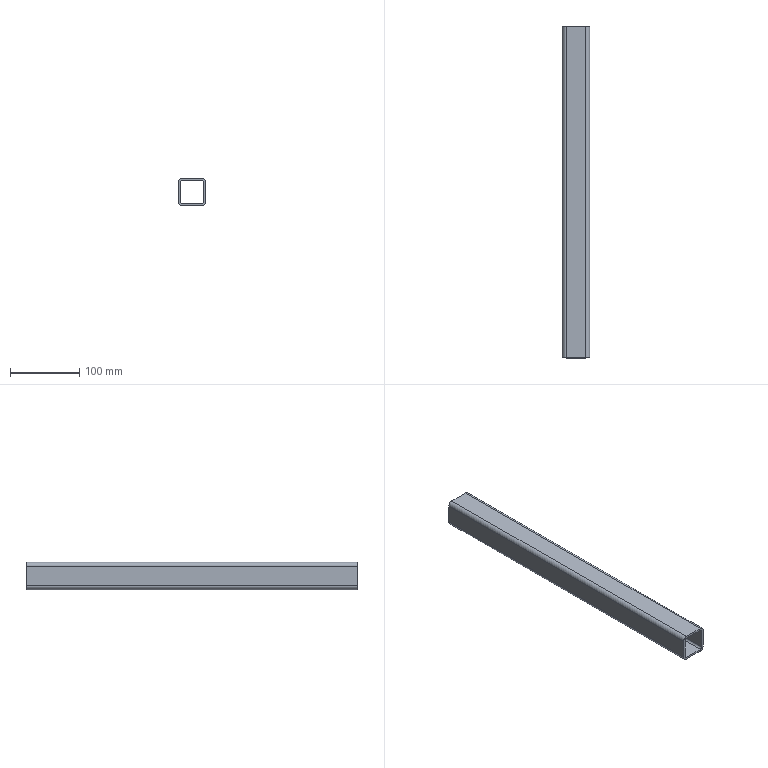Part | SolidWorks | features WeldMemberFeat 1, WeldmentFeature 1 | 1 solid | 18 faces | box 40 x 480 x 40 mm | volume 201995 mm3 | plane 10 | cylinder 8 | commonest cylinder face diameters 6 x4 12 x4
STEP:
#1=CARTESIAN_POINT('',(-20.,0.,14.));
#2=VERTEX_POINT('',#1);
#3=CARTESIAN_POINT('',(-14.,0.,20.));
#4=VERTEX_POINT('',#3);
#5=CARTESIAN_POINT('',(-14.,0.,14.));
#6=DIRECTION('',(0.,1.,0.));
#7=DIRECTION('',(0.,0.,1.));
#8=AXIS2_PLACEMENT_3D('',#5,#6,#7);
#9=CIRCLE('',#8,6.);
#10=EDGE_CURVE('',#2,#4,#9,.T.);
#11=ORIENTED_EDGE('',*,*,#10,.T.);
#12=CARTESIAN_POINT('',(-14.,480.,20.));
#13=VERTEX_POINT('',#12);
#14=CARTESIAN_POINT('',(-14.,480.,20.));
#15=DIRECTION('',(0.,-1.,0.));
#16=VECTOR('',#15,1000.);
#17=LINE('',#14,#16);
#18=EDGE_CURVE('',#13,#4,#17,.T.);
#19=ORIENTED_EDGE('',*,*,#18,.F.);
#20=CARTESIAN_POINT('',(-20.,480.,14.));
#21=VERTEX_POINT('',#20);
#22=CARTESIAN_POINT('',(-14.,480.,14.));
#23=DIRECTION('',(0.,1.,0.));
#24=DIRECTION('',(0.,0.,1.));
#25=AXIS2_PLACEMENT_3D('',#22,#23,#24);
#26=CIRCLE('',#25,6.);
#27=EDGE_CURVE('',#21,#13,#26,.T.);
#28=ORIENTED_EDGE('',*,*,#27,.F.);
#29=CARTESIAN_POINT('',(-20.,480.,14.));
#30=DIRECTION('',(0.,-1.,0.));
#31=VECTOR('',#30,1000.);
#32=LINE('',#29,#31);
#33=EDGE_CURVE('',#21,#2,#32,.T.);
#34=ORIENTED_EDGE('',*,*,#33,.T.);
#35=EDGE_LOOP('',(#11,#19,#28,#34));
#36=FACE_OUTER_BOUND('',#35,.T.);
#37=CARTESIAN_POINT('',(-14.,480.,14.));
#38=DIRECTION('',(0.,-1.,0.));
#39=DIRECTION('',(0.,0.,-1.));
#40=AXIS2_PLACEMENT_3D('',#37,#38,#39);
#41=CYLINDRICAL_SURFACE('',#40,6.);
#42=ADVANCED_FACE('',(#36),#41,.T.);
#43=CARTESIAN_POINT('',(14.,0.,20.));
#44=VERTEX_POINT('',#43);
#45=CARTESIAN_POINT('',(-14.,0.,20.));
#46=DIRECTION('',(1.,0.,0.));
#47=VECTOR('',#46,1000.);
#48=LINE('',#45,#47);
#49=EDGE_CURVE('',#4,#44,#48,.T.);
#50=ORIENTED_EDGE('',*,*,#49,.T.);
#51=CARTESIAN_POINT('',(14.,480.,20.));
#52=VERTEX_POINT('',#51);
#53=CARTESIAN_POINT('',(14.,480.,20.));
#54=DIRECTION('',(0.,-1.,0.));
#55=VECTOR('',#54,1000.);
#56=LINE('',#53,#55);
#57=EDGE_CURVE('',#52,#44,#56,.T.);
#58=ORIENTED_EDGE('',*,*,#57,.F.);
#59=CARTESIAN_POINT('',(-14.,480.,20.));
#60=DIRECTION('',(1.,0.,0.));
#61=VECTOR('',#60,1000.);
#62=LINE('',#59,#61);
#63=EDGE_CURVE('',#13,#52,#62,.T.);
#64=ORIENTED_EDGE('',*,*,#63,.F.);
#65=ORIENTED_EDGE('',*,*,#18,.T.);
#66=EDGE_LOOP('',(#50,#58,#64,#65));
#67=FACE_OUTER_BOUND('',#66,.T.);
#68=CARTESIAN_POINT('',(-14.,480.,20.));
#69=DIRECTION('',(0.,0.,-1.));
#70=DIRECTION('',(-1.,0.,0.));
#71=AXIS2_PLACEMENT_3D('',#68,#69,#70);
#72=PLANE('',#71);
#73=ADVANCED_FACE('',(#67),#72,.F.);
#74=CARTESIAN_POINT('',(20.,0.,14.));
#75=VERTEX_POINT('',#74);
#76=CARTESIAN_POINT('',(14.,0.,14.));
#77=DIRECTION('',(0.,1.,0.));
#78=DIRECTION('',(0.,0.,1.));
#79=AXIS2_PLACEMENT_3D('',#76,#77,#78);
#80=CIRCLE('',#79,6.);
#81=EDGE_CURVE('',#44,#75,#80,.T.);
#82=ORIENTED_EDGE('',*,*,#81,.T.);
#83=CARTESIAN_POINT('',(20.,480.,14.));
#84=VERTEX_POINT('',#83);
#85=CARTESIAN_POINT('',(20.,480.,14.));
#86=DIRECTION('',(0.,-1.,0.));
#87=VECTOR('',#86,1000.);
#88=LINE('',#85,#87);
#89=EDGE_CURVE('',#84,#75,#88,.T.);
#90=ORIENTED_EDGE('',*,*,#89,.F.);
#91=CARTESIAN_POINT('',(14.,480.,14.));
#92=DIRECTION('',(0.,1.,0.));
#93=DIRECTION('',(0.,0.,1.));
#94=AXIS2_PLACEMENT_3D('',#91,#92,#93);
#95=CIRCLE('',#94,6.);
#96=EDGE_CURVE('',#52,#84,#95,.T.);
#97=ORIENTED_EDGE('',*,*,#96,.F.);
#98=ORIENTED_EDGE('',*,*,#57,.T.);
#99=EDGE_LOOP('',(#82,#90,#97,#98));
#100=FACE_OUTER_BOUND('',#99,.T.);
#101=CARTESIAN_POINT('',(14.,480.,14.));
#102=DIRECTION('',(0.,-1.,0.));
#103=DIRECTION('',(0.,0.,-1.));
#104=AXIS2_PLACEMENT_3D('',#101,#102,#103);
#105=CYLINDRICAL_SURFACE('',#104,6.);
#106=ADVANCED_FACE('',(#100),#105,.T.);
#107=CARTESIAN_POINT('',(20.,0.,-14.));
#108=VERTEX_POINT('',#107);
#109=CARTESIAN_POINT('',(20.,0.,-14.));
#110=DIRECTION('',(0.,0.,-1.));
#111=VECTOR('',#110,1000.);
#112=LINE('',#109,#111);
#113=EDGE_CURVE('',#75,#108,#112,.T.);
#114=ORIENTED_EDGE('',*,*,#113,.T.);
#115=CARTESIAN_POINT('',(20.,480.,-14.));
#116=VERTEX_POINT('',#115);
#117=CARTESIAN_POINT('',(20.,480.,-14.));
#118=DIRECTION('',(0.,-1.,0.));
#119=VECTOR('',#118,1000.);
#120=LINE('',#117,#119);
#121=EDGE_CURVE('',#116,#108,#120,.T.);
#122=ORIENTED_EDGE('',*,*,#121,.F.);
#123=CARTESIAN_POINT('',(20.,480.,-14.));
#124=DIRECTION('',(0.,0.,-1.));
#125=VECTOR('',#124,1000.);
#126=LINE('',#123,#125);
#127=EDGE_CURVE('',#84,#116,#126,.T.);
#128=ORIENTED_EDGE('',*,*,#127,.F.);
#129=ORIENTED_EDGE('',*,*,#89,.T.);
#130=EDGE_LOOP('',(#114,#122,#128,#129));
#131=FACE_OUTER_BOUND('',#130,.T.);
#132=CARTESIAN_POINT('',(20.,480.,-14.));
#133=DIRECTION('',(-1.,0.,0.));
#134=DIRECTION('',(0.,0.,1.));
#135=AXIS2_PLACEMENT_3D('',#132,#133,#134);
#136=PLANE('',#135);
#137=ADVANCED_FACE('',(#131),#136,.F.);
#138=CARTESIAN_POINT('',(14.,0.,-20.));
#139=VERTEX_POINT('',#138);
#140=CARTESIAN_POINT('',(14.,0.,-14.));
#141=DIRECTION('',(0.,1.,0.));
#142=DIRECTION('',(0.,0.,1.));
#143=AXIS2_PLACEMENT_3D('',#140,#141,#142);
#144=CIRCLE('',#143,6.);
#145=EDGE_CURVE('',#108,#139,#144,.T.);
#146=ORIENTED_EDGE('',*,*,#145,.T.);
#147=CARTESIAN_POINT('',(14.,480.,-20.));
#148=VERTEX_POINT('',#147);
#149=CARTESIAN_POINT('',(14.,480.,-20.));
#150=DIRECTION('',(0.,-1.,0.));
#151=VECTOR('',#150,1000.);
#152=LINE('',#149,#151);
#153=EDGE_CURVE('',#148,#139,#152,.T.);
#154=ORIENTED_EDGE('',*,*,#153,.F.);
#155=CARTESIAN_POINT('',(14.,480.,-14.));
#156=DIRECTION('',(0.,1.,0.));
#157=DIRECTION('',(0.,0.,1.));
#158=AXIS2_PLACEMENT_3D('',#155,#156,#157);
#159=CIRCLE('',#158,6.);
#160=EDGE_CURVE('',#116,#148,#159,.T.);
#161=ORIENTED_EDGE('',*,*,#160,.F.);
#162=ORIENTED_EDGE('',*,*,#121,.T.);
#163=EDGE_LOOP('',(#146,#154,#161,#162));
#164=FACE_OUTER_BOUND('',#163,.T.);
#165=CARTESIAN_POINT('',(14.,480.,-14.));
#166=DIRECTION('',(0.,-1.,0.));
#167=DIRECTION('',(0.,0.,-1.));
#168=AXIS2_PLACEMENT_3D('',#165,#166,#167);
#169=CYLINDRICAL_SURFACE('',#168,6.);
#170=ADVANCED_FACE('',(#164),#169,.T.);
#171=CARTESIAN_POINT('',(-14.,0.,-20.));
#172=VERTEX_POINT('',#171);
#173=CARTESIAN_POINT('',(14.,0.,-20.));
#174=DIRECTION('',(-1.,0.,0.));
#175=VECTOR('',#174,1000.);
#176=LINE('',#173,#175);
#177=EDGE_CURVE('',#139,#172,#176,.T.);
#178=ORIENTED_EDGE('',*,*,#177,.T.);
#179=CARTESIAN_POINT('',(-14.,480.,-20.));
#180=VERTEX_POINT('',#179);
#181=CARTESIAN_POINT('',(-14.,480.,-20.));
#182=DIRECTION('',(0.,-1.,0.));
#183=VECTOR('',#182,1000.);
#184=LINE('',#181,#183);
#185=EDGE_CURVE('',#180,#172,#184,.T.);
#186=ORIENTED_EDGE('',*,*,#185,.F.);
#187=CARTESIAN_POINT('',(14.,480.,-20.));
#188=DIRECTION('',(-1.,0.,0.));
#189=VECTOR('',#188,1000.);
#190=LINE('',#187,#189);
#191=EDGE_CURVE('',#148,#180,#190,.T.);
#192=ORIENTED_EDGE('',*,*,#191,.F.);
#193=ORIENTED_EDGE('',*,*,#153,.T.);
#194=EDGE_LOOP('',(#178,#186,#192,#193));
#195=FACE_OUTER_BOUND('',#194,.T.);
#196=CARTESIAN_POINT('',(14.,480.,-20.));
#197=DIRECTION('',(0.,0.,1.));
#198=DIRECTION('',(1.,0.,0.));
#199=AXIS2_PLACEMENT_3D('',#196,#197,#198);
#200=PLANE('',#199);
#201=ADVANCED_FACE('',(#195),#200,.F.);
#202=CARTESIAN_POINT('',(-20.,0.,-14.));
#203=VERTEX_POINT('',#202);
#204=CARTESIAN_POINT('',(-14.,0.,-14.));
#205=DIRECTION('',(0.,1.,0.));
#206=DIRECTION('',(0.,0.,1.));
#207=AXIS2_PLACEMENT_3D('',#204,#205,#206);
#208=CIRCLE('',#207,6.);
#209=EDGE_CURVE('',#172,#203,#208,.T.);
#210=ORIENTED_EDGE('',*,*,#209,.T.);
#211=CARTESIAN_POINT('',(-20.,480.,-14.));
#212=VERTEX_POINT('',#211);
#213=CARTESIAN_POINT('',(-20.,480.,-14.));
#214=DIRECTION('',(0.,-1.,0.));
#215=VECTOR('',#214,1000.);
#216=LINE('',#213,#215);
#217=EDGE_CURVE('',#212,#203,#216,.T.);
#218=ORIENTED_EDGE('',*,*,#217,.F.);
#219=CARTESIAN_POINT('',(-14.,480.,-14.));
#220=DIRECTION('',(0.,1.,0.));
#221=DIRECTION('',(0.,0.,1.));
#222=AXIS2_PLACEMENT_3D('',#219,#220,#221);
#223=CIRCLE('',#222,6.);
#224=EDGE_CURVE('',#180,#212,#223,.T.);
#225=ORIENTED_EDGE('',*,*,#224,.F.);
#226=ORIENTED_EDGE('',*,*,#185,.T.);
#227=EDGE_LOOP('',(#210,#218,#225,#226));
#228=FACE_OUTER_BOUND('',#227,.T.);
#229=CARTESIAN_POINT('',(-14.,480.,-14.));
#230=DIRECTION('',(0.,-1.,0.));
#231=DIRECTION('',(0.,0.,-1.));
#232=AXIS2_PLACEMENT_3D('',#229,#230,#231);
#233=CYLINDRICAL_SURFACE('',#232,6.);
#234=ADVANCED_FACE('',(#228),#233,.T.);
#235=CARTESIAN_POINT('',(14.,0.,17.));
#236=VERTEX_POINT('',#235);
#237=CARTESIAN_POINT('',(17.,0.,14.));
#238=VERTEX_POINT('',#237);
#239=CARTESIAN_POINT('',(14.,0.,14.));
#240=DIRECTION('',(0.,1.,0.));
#241=DIRECTION('',(0.,0.,1.));
#242=AXIS2_PLACEMENT_3D('',#239,#240,#241);
#243=CIRCLE('',#242,3.);
#244=EDGE_CURVE('',#236,#238,#243,.T.);
#245=ORIENTED_EDGE('',*,*,#244,.F.);
#246=CARTESIAN_POINT('',(14.,480.,17.));
#247=VERTEX_POINT('',#246);
#248=CARTESIAN_POINT('',(14.,480.,17.));
#249=DIRECTION('',(0.,-1.,0.));
#250=VECTOR('',#249,1000.);
#251=LINE('',#248,#250);
#252=EDGE_CURVE('',#247,#236,#251,.T.);
#253=ORIENTED_EDGE('',*,*,#252,.F.);
#254=CARTESIAN_POINT('',(17.,480.,14.));
#255=VERTEX_POINT('',#254);
#256=CARTESIAN_POINT('',(14.,480.,14.));
#257=DIRECTION('',(0.,1.,0.));
#258=DIRECTION('',(0.,0.,1.));
#259=AXIS2_PLACEMENT_3D('',#256,#257,#258);
#260=CIRCLE('',#259,3.);
#261=EDGE_CURVE('',#247,#255,#260,.T.);
#262=ORIENTED_EDGE('',*,*,#261,.T.);
#263=CARTESIAN_POINT('',(17.,480.,14.));
#264=DIRECTION('',(0.,-1.,0.));
#265=VECTOR('',#264,1000.);
#266=LINE('',#263,#265);
#267=EDGE_CURVE('',#255,#238,#266,.T.);
#268=ORIENTED_EDGE('',*,*,#267,.T.);
#269=EDGE_LOOP('',(#245,#253,#262,#268));
#270=FACE_OUTER_BOUND('',#269,.T.);
#271=CARTESIAN_POINT('',(14.,480.,14.));
#272=DIRECTION('',(0.,-1.,0.));
#273=DIRECTION('',(0.,0.,-1.));
#274=AXIS2_PLACEMENT_3D('',#271,#272,#273);
#275=CYLINDRICAL_SURFACE('',#274,3.);
#276=ADVANCED_FACE('',(#270),#275,.F.);
#277=CARTESIAN_POINT('',(-14.,0.,17.));
#278=VERTEX_POINT('',#277);
#279=CARTESIAN_POINT('',(-14.,0.,17.));
#280=DIRECTION('',(1.,0.,0.));
#281=VECTOR('',#280,1000.);
#282=LINE('',#279,#281);
#283=EDGE_CURVE('',#278,#236,#282,.T.);
#284=ORIENTED_EDGE('',*,*,#283,.F.);
#285=CARTESIAN_POINT('',(-14.,480.,17.));
#286=VERTEX_POINT('',#285);
#287=CARTESIAN_POINT('',(-14.,480.,17.));
#288=DIRECTION('',(0.,-1.,0.));
#289=VECTOR('',#288,1000.);
#290=LINE('',#287,#289);
#291=EDGE_CURVE('',#286,#278,#290,.T.);
#292=ORIENTED_EDGE('',*,*,#291,.F.);
#293=CARTESIAN_POINT('',(-14.,480.,17.));
#294=DIRECTION('',(1.,0.,0.));
#295=VECTOR('',#294,1000.);
#296=LINE('',#293,#295);
#297=EDGE_CURVE('',#286,#247,#296,.T.);
#298=ORIENTED_EDGE('',*,*,#297,.T.);
#299=ORIENTED_EDGE('',*,*,#252,.T.);
#300=EDGE_LOOP('',(#284,#292,#298,#299));
#301=FACE_OUTER_BOUND('',#300,.T.);
#302=CARTESIAN_POINT('',(-14.,480.,17.));
#303=DIRECTION('',(0.,0.,-1.));
#304=DIRECTION('',(-1.,0.,0.));
#305=AXIS2_PLACEMENT_3D('',#302,#303,#304);
#306=PLANE('',#305);
#307=ADVANCED_FACE('',(#301),#306,.T.);
#308=CARTESIAN_POINT('',(-17.,0.,14.));
#309=VERTEX_POINT('',#308);
#310=CARTESIAN_POINT('',(-14.,0.,14.));
#311=DIRECTION('',(0.,1.,0.));
#312=DIRECTION('',(0.,0.,1.));
#313=AXIS2_PLACEMENT_3D('',#310,#311,#312);
#314=CIRCLE('',#313,3.);
#315=EDGE_CURVE('',#309,#278,#314,.T.);
#316=ORIENTED_EDGE('',*,*,#315,.F.);
#317=CARTESIAN_POINT('',(-17.,480.,14.));
#318=VERTEX_POINT('',#317);
#319=CARTESIAN_POINT('',(-17.,480.,14.));
#320=DIRECTION('',(0.,-1.,0.));
#321=VECTOR('',#320,1000.);
#322=LINE('',#319,#321);
#323=EDGE_CURVE('',#318,#309,#322,.T.);
#324=ORIENTED_EDGE('',*,*,#323,.F.);
#325=CARTESIAN_POINT('',(-14.,480.,14.));
#326=DIRECTION('',(0.,1.,0.));
#327=DIRECTION('',(0.,0.,1.));
#328=AXIS2_PLACEMENT_3D('',#325,#326,#327);
#329=CIRCLE('',#328,3.);
#330=EDGE_CURVE('',#318,#286,#329,.T.);
#331=ORIENTED_EDGE('',*,*,#330,.T.);
#332=ORIENTED_EDGE('',*,*,#291,.T.);
#333=EDGE_LOOP('',(#316,#324,#331,#332));
#334=FACE_OUTER_BOUND('',#333,.T.);
#335=CARTESIAN_POINT('',(-14.,480.,14.));
#336=DIRECTION('',(0.,-1.,0.));
#337=DIRECTION('',(0.,0.,-1.));
#338=AXIS2_PLACEMENT_3D('',#335,#336,#337);
#339=CYLINDRICAL_SURFACE('',#338,3.);
#340=ADVANCED_FACE('',(#334),#339,.F.);
#341=CARTESIAN_POINT('',(-17.,0.,-14.));
#342=VERTEX_POINT('',#341);
#343=CARTESIAN_POINT('',(-17.,0.,14.));
#344=DIRECTION('',(0.,0.,1.));
#345=VECTOR('',#344,1000.);
#346=LINE('',#343,#345);
#347=EDGE_CURVE('',#342,#309,#346,.T.);
#348=ORIENTED_EDGE('',*,*,#347,.F.);
#349=CARTESIAN_POINT('',(-17.,480.,-14.));
#350=VERTEX_POINT('',#349);
#351=CARTESIAN_POINT('',(-17.,480.,-14.));
#352=DIRECTION('',(0.,-1.,0.));
#353=VECTOR('',#352,1000.);
#354=LINE('',#351,#353);
#355=EDGE_CURVE('',#350,#342,#354,.T.);
#356=ORIENTED_EDGE('',*,*,#355,.F.);
#357=CARTESIAN_POINT('',(-17.,480.,14.));
#358=DIRECTION('',(0.,0.,1.));
#359=VECTOR('',#358,1000.);
#360=LINE('',#357,#359);
#361=EDGE_CURVE('',#350,#318,#360,.T.);
#362=ORIENTED_EDGE('',*,*,#361,.T.);
#363=ORIENTED_EDGE('',*,*,#323,.T.);
#364=EDGE_LOOP('',(#348,#356,#362,#363));
#365=FACE_OUTER_BOUND('',#364,.T.);
#366=CARTESIAN_POINT('',(-17.,480.,14.));
#367=DIRECTION('',(1.,0.,0.));
#368=DIRECTION('',(0.,0.,-1.));
#369=AXIS2_PLACEMENT_3D('',#366,#367,#368);
#370=PLANE('',#369);
#371=ADVANCED_FACE('',(#365),#370,.T.);
#372=CARTESIAN_POINT('',(-14.,0.,-17.));
#373=VERTEX_POINT('',#372);
#374=CARTESIAN_POINT('',(-14.,0.,-14.));
#375=DIRECTION('',(0.,1.,0.));
#376=DIRECTION('',(0.,0.,1.));
#377=AXIS2_PLACEMENT_3D('',#374,#375,#376);
#378=CIRCLE('',#377,3.);
#379=EDGE_CURVE('',#373,#342,#378,.T.);
#380=ORIENTED_EDGE('',*,*,#379,.F.);
#381=CARTESIAN_POINT('',(-14.,480.,-17.));
#382=VERTEX_POINT('',#381);
#383=CARTESIAN_POINT('',(-14.,480.,-17.));
#384=DIRECTION('',(0.,-1.,0.));
#385=VECTOR('',#384,1000.);
#386=LINE('',#383,#385);
#387=EDGE_CURVE('',#382,#373,#386,.T.);
#388=ORIENTED_EDGE('',*,*,#387,.F.);
#389=CARTESIAN_POINT('',(-14.,480.,-14.));
#390=DIRECTION('',(0.,1.,0.));
#391=DIRECTION('',(0.,0.,1.));
#392=AXIS2_PLACEMENT_3D('',#389,#390,#391);
#393=CIRCLE('',#392,3.);
#394=EDGE_CURVE('',#382,#350,#393,.T.);
#395=ORIENTED_EDGE('',*,*,#394,.T.);
#396=ORIENTED_EDGE('',*,*,#355,.T.);
#397=EDGE_LOOP('',(#380,#388,#395,#396));
#398=FACE_OUTER_BOUND('',#397,.T.);
#399=CARTESIAN_POINT('',(-14.,480.,-14.));
#400=DIRECTION('',(0.,-1.,0.));
#401=DIRECTION('',(0.,0.,-1.));
#402=AXIS2_PLACEMENT_3D('',#399,#400,#401);
#403=CYLINDRICAL_SURFACE('',#402,3.);
#404=ADVANCED_FACE('',(#398),#403,.F.);
#405=CARTESIAN_POINT('',(14.,0.,-17.));
#406=VERTEX_POINT('',#405);
#407=CARTESIAN_POINT('',(14.,0.,-17.));
#408=DIRECTION('',(-1.,0.,0.));
#409=VECTOR('',#408,1000.);
#410=LINE('',#407,#409);
#411=EDGE_CURVE('',#406,#373,#410,.T.);
#412=ORIENTED_EDGE('',*,*,#411,.F.);
#413=CARTESIAN_POINT('',(14.,480.,-17.));
#414=VERTEX_POINT('',#413);
#415=CARTESIAN_POINT('',(14.,480.,-17.));
#416=DIRECTION('',(0.,-1.,0.));
#417=VECTOR('',#416,1000.);
#418=LINE('',#415,#417);
#419=EDGE_CURVE('',#414,#406,#418,.T.);
#420=ORIENTED_EDGE('',*,*,#419,.F.);
#421=CARTESIAN_POINT('',(14.,480.,-17.));
#422=DIRECTION('',(-1.,0.,0.));
#423=VECTOR('',#422,1000.);
#424=LINE('',#421,#423);
#425=EDGE_CURVE('',#414,#382,#424,.T.);
#426=ORIENTED_EDGE('',*,*,#425,.T.);
#427=ORIENTED_EDGE('',*,*,#387,.T.);
#428=EDGE_LOOP('',(#412,#420,#426,#427));
#429=FACE_OUTER_BOUND('',#428,.T.);
#430=CARTESIAN_POINT('',(14.,480.,-17.));
#431=DIRECTION('',(0.,0.,1.));
#432=DIRECTION('',(1.,0.,0.));
#433=AXIS2_PLACEMENT_3D('',#430,#431,#432);
#434=PLANE('',#433);
#435=ADVANCED_FACE('',(#429),#434,.T.);
#436=CARTESIAN_POINT('',(17.,0.,-14.));
#437=VERTEX_POINT('',#436);
#438=CARTESIAN_POINT('',(14.,0.,-14.));
#439=DIRECTION('',(0.,1.,0.));
#440=DIRECTION('',(0.,0.,1.));
#441=AXIS2_PLACEMENT_3D('',#438,#439,#440);
#442=CIRCLE('',#441,3.);
#443=EDGE_CURVE('',#437,#406,#442,.T.);
#444=ORIENTED_EDGE('',*,*,#443,.F.);
#445=CARTESIAN_POINT('',(17.,480.,-14.));
#446=VERTEX_POINT('',#445);
#447=CARTESIAN_POINT('',(17.,480.,-14.));
#448=DIRECTION('',(0.,-1.,0.));
#449=VECTOR('',#448,1000.);
#450=LINE('',#447,#449);
#451=EDGE_CURVE('',#446,#437,#450,.T.);
#452=ORIENTED_EDGE('',*,*,#451,.F.);
#453=CARTESIAN_POINT('',(14.,480.,-14.));
#454=DIRECTION('',(0.,1.,0.));
#455=DIRECTION('',(0.,0.,1.));
#456=AXIS2_PLACEMENT_3D('',#453,#454,#455);
#457=CIRCLE('',#456,3.);
#458=EDGE_CURVE('',#446,#414,#457,.T.);
#459=ORIENTED_EDGE('',*,*,#458,.T.);
#460=ORIENTED_EDGE('',*,*,#419,.T.);
#461=EDGE_LOOP('',(#444,#452,#459,#460));
#462=FACE_OUTER_BOUND('',#461,.T.);
#463=CARTESIAN_POINT('',(14.,480.,-14.));
#464=DIRECTION('',(0.,-1.,0.));
#465=DIRECTION('',(0.,0.,-1.));
#466=AXIS2_PLACEMENT_3D('',#463,#464,#465);
#467=CYLINDRICAL_SURFACE('',#466,3.);
#468=ADVANCED_FACE('',(#462),#467,.F.);
#469=CARTESIAN_POINT('',(17.,0.,-14.));
#470=DIRECTION('',(0.,0.,-1.));
#471=VECTOR('',#470,1000.);
#472=LINE('',#469,#471);
#473=EDGE_CURVE('',#238,#437,#472,.T.);
#474=ORIENTED_EDGE('',*,*,#473,.F.);
#475=ORIENTED_EDGE('',*,*,#267,.F.);
#476=CARTESIAN_POINT('',(17.,480.,-14.));
#477=DIRECTION('',(0.,0.,-1.));
#478=VECTOR('',#477,1000.);
#479=LINE('',#476,#478);
#480=EDGE_CURVE('',#255,#446,#479,.T.);
#481=ORIENTED_EDGE('',*,*,#480,.T.);
#482=ORIENTED_EDGE('',*,*,#451,.T.);
#483=EDGE_LOOP('',(#474,#475,#481,#482));
#484=FACE_OUTER_BOUND('',#483,.T.);
#485=CARTESIAN_POINT('',(17.,480.,-14.));
#486=DIRECTION('',(-1.,0.,0.));
#487=DIRECTION('',(0.,0.,1.));
#488=AXIS2_PLACEMENT_3D('',#485,#486,#487);
#489=PLANE('',#488);
#490=ADVANCED_FACE('',(#484),#489,.T.);
#491=CARTESIAN_POINT('',(-20.,0.,14.));
#492=DIRECTION('',(0.,0.,1.));
#493=VECTOR('',#492,1000.);
#494=LINE('',#491,#493);
#495=EDGE_CURVE('',#203,#2,#494,.T.);
#496=ORIENTED_EDGE('',*,*,#495,.T.);
#497=ORIENTED_EDGE('',*,*,#33,.F.);
#498=CARTESIAN_POINT('',(-20.,480.,14.));
#499=DIRECTION('',(0.,0.,1.));
#500=VECTOR('',#499,1000.);
#501=LINE('',#498,#500);
#502=EDGE_CURVE('',#212,#21,#501,.T.);
#503=ORIENTED_EDGE('',*,*,#502,.F.);
#504=ORIENTED_EDGE('',*,*,#217,.T.);
#505=EDGE_LOOP('',(#496,#497,#503,#504));
#506=FACE_OUTER_BOUND('',#505,.T.);
#507=CARTESIAN_POINT('',(-20.,480.,14.));
#508=DIRECTION('',(1.,0.,0.));
#509=DIRECTION('',(0.,0.,-1.));
#510=AXIS2_PLACEMENT_3D('',#507,#508,#509);
#511=PLANE('',#510);
#512=ADVANCED_FACE('',(#506),#511,.F.);
#513=ORIENTED_EDGE('',*,*,#261,.F.);
#514=ORIENTED_EDGE('',*,*,#297,.F.);
#515=ORIENTED_EDGE('',*,*,#330,.F.);
#516=ORIENTED_EDGE('',*,*,#361,.F.);
#517=ORIENTED_EDGE('',*,*,#394,.F.);
#518=ORIENTED_EDGE('',*,*,#425,.F.);
#519=ORIENTED_EDGE('',*,*,#458,.F.);
#520=ORIENTED_EDGE('',*,*,#480,.F.);
#521=EDGE_LOOP('',(#513,#514,#515,#516,#517,#518,#519,#520));
#522=FACE_BOUND('',#521,.T.);
#523=ORIENTED_EDGE('',*,*,#27,.T.);
#524=ORIENTED_EDGE('',*,*,#63,.T.);
#525=ORIENTED_EDGE('',*,*,#96,.T.);
#526=ORIENTED_EDGE('',*,*,#127,.T.);
#527=ORIENTED_EDGE('',*,*,#160,.T.);
#528=ORIENTED_EDGE('',*,*,#191,.T.);
#529=ORIENTED_EDGE('',*,*,#224,.T.);
#530=ORIENTED_EDGE('',*,*,#502,.T.);
#531=EDGE_LOOP('',(#523,#524,#525,#526,#527,#528,#529,#530));
#532=FACE_OUTER_BOUND('',#531,.T.);
#533=CARTESIAN_POINT('',(-14.,480.,14.));
#534=DIRECTION('',(0.,1.,0.));
#535=DIRECTION('',(0.,0.,1.));
#536=AXIS2_PLACEMENT_3D('',#533,#534,#535);
#537=PLANE('',#536);
#538=ADVANCED_FACE('',(#522,#532),#537,.T.);
#539=ORIENTED_EDGE('',*,*,#244,.T.);
#540=ORIENTED_EDGE('',*,*,#473,.T.);
#541=ORIENTED_EDGE('',*,*,#443,.T.);
#542=ORIENTED_EDGE('',*,*,#411,.T.);
#543=ORIENTED_EDGE('',*,*,#379,.T.);
#544=ORIENTED_EDGE('',*,*,#347,.T.);
#545=ORIENTED_EDGE('',*,*,#315,.T.);
#546=ORIENTED_EDGE('',*,*,#283,.T.);
#547=EDGE_LOOP('',(#539,#540,#541,#542,#543,#544,#545,#546));
#548=FACE_BOUND('',#547,.T.);
#549=ORIENTED_EDGE('',*,*,#10,.F.);
#550=ORIENTED_EDGE('',*,*,#495,.F.);
#551=ORIENTED_EDGE('',*,*,#209,.F.);
#552=ORIENTED_EDGE('',*,*,#177,.F.);
#553=ORIENTED_EDGE('',*,*,#145,.F.);
#554=ORIENTED_EDGE('',*,*,#113,.F.);
#555=ORIENTED_EDGE('',*,*,#81,.F.);
#556=ORIENTED_EDGE('',*,*,#49,.F.);
#557=EDGE_LOOP('',(#549,#550,#551,#552,#553,#554,#555,#556));
#558=FACE_OUTER_BOUND('',#557,.T.);
#559=CARTESIAN_POINT('',(-14.,0.,14.));
#560=DIRECTION('',(0.,1.,0.));
#561=DIRECTION('',(0.,0.,1.));
#562=AXIS2_PLACEMENT_3D('',#559,#560,#561);
#563=PLANE('',#562);
#564=ADVANCED_FACE('',(#548,#558),#563,.F.);
#565=CLOSED_SHELL('',(#42,#73,#106,#137,#170,#201,#234,#276,#307,#340,#371,#404,#435,#468,#490,#512,#538,#564));
#566=MANIFOLD_SOLID_BREP('',#565);
#567=CARTESIAN_POINT('',(0.,0.,0.));
#568=DIRECTION('',(0.,0.,1.));
#569=DIRECTION('',(1.,0.,0.));
#570=AXIS2_PLACEMENT_3D('',#567,#568,#569);
#571=(LENGTH_UNIT()NAMED_UNIT(*)SI_UNIT(.MILLI.,.METRE.));
#572=UNCERTAINTY_MEASURE_WITH_UNIT(LENGTH_MEASURE(0.00001),#571,'','');
#573=(NAMED_UNIT(*)PLANE_ANGLE_UNIT()SI_UNIT($,.RADIAN.));
#574=(NAMED_UNIT(*)SI_UNIT($,.STERADIAN.)SOLID_ANGLE_UNIT());
#575=(GEOMETRIC_REPRESENTATION_CONTEXT(3)GLOBAL_UNCERTAINTY_ASSIGNED_CONTEXT((#572))GLOBAL_UNIT_ASSIGNED_CONTEXT((#571,#573,#574))REPRESENTATION_CONTEXT('',''));
#576=ADVANCED_BREP_SHAPE_REPRESENTATION('',(#566,#570),#575);